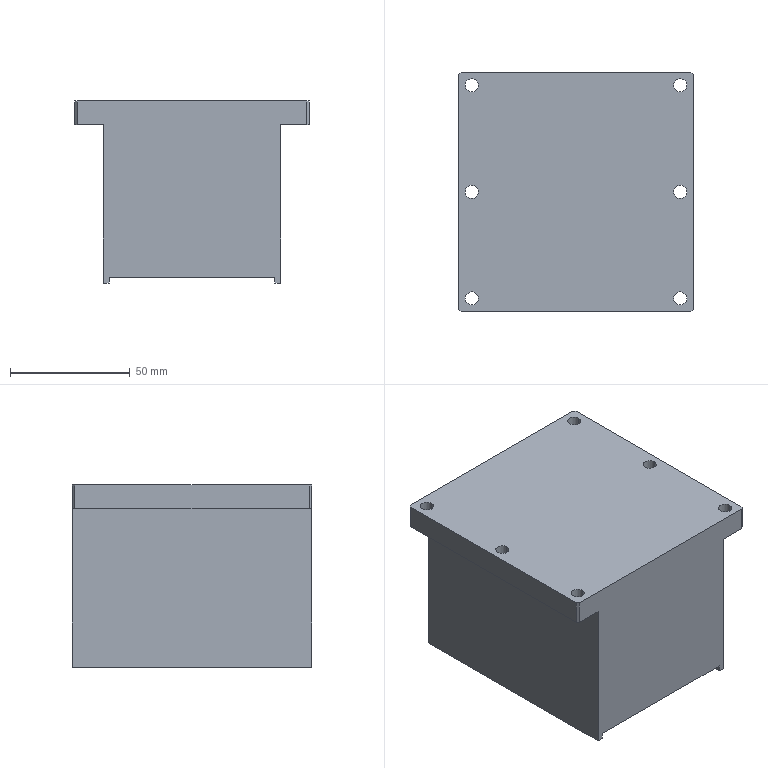Part | STEP file | 11-FG-S00811 | 1 solid | 70 faces | box 98 x 100 x 76 mm | volume 565928 mm3 | cylinder 32 | cone 20 | plane 18 | commonest cylinder face diameters 4.2 x20 5.5 x12